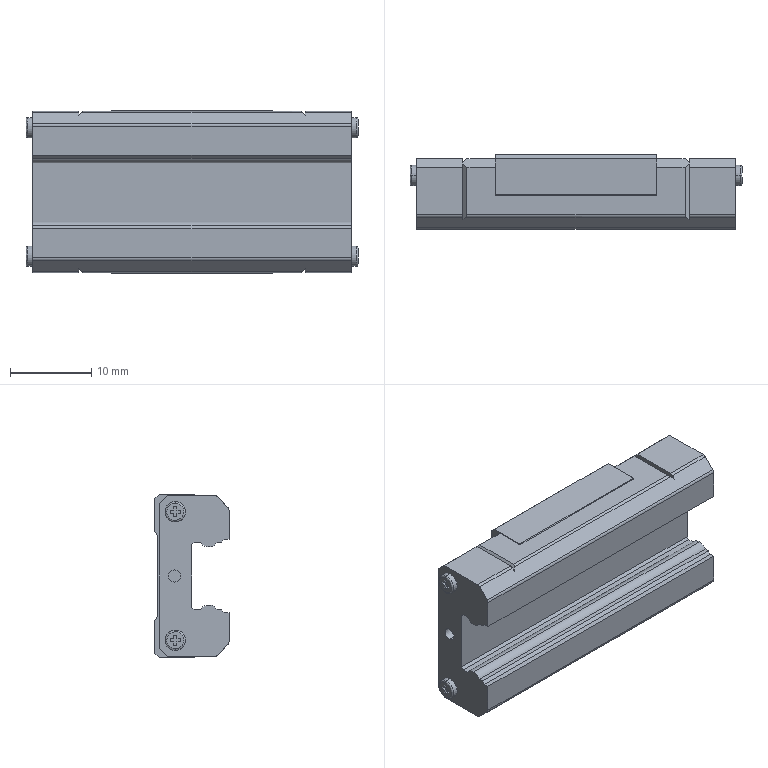Part | STEP file | qnSceond_SRS9MQZUU Slider | 1 solid | 178 faces | box 40.8 x 9.1 x 20 mm | volume 5179 mm3 | plane 118 | cylinder 36 | cone 16 | spline 8 | commonest cylinder face diameters 1 x10 2.459 x8 2.5 x8 2.2 x6 1.5 x4